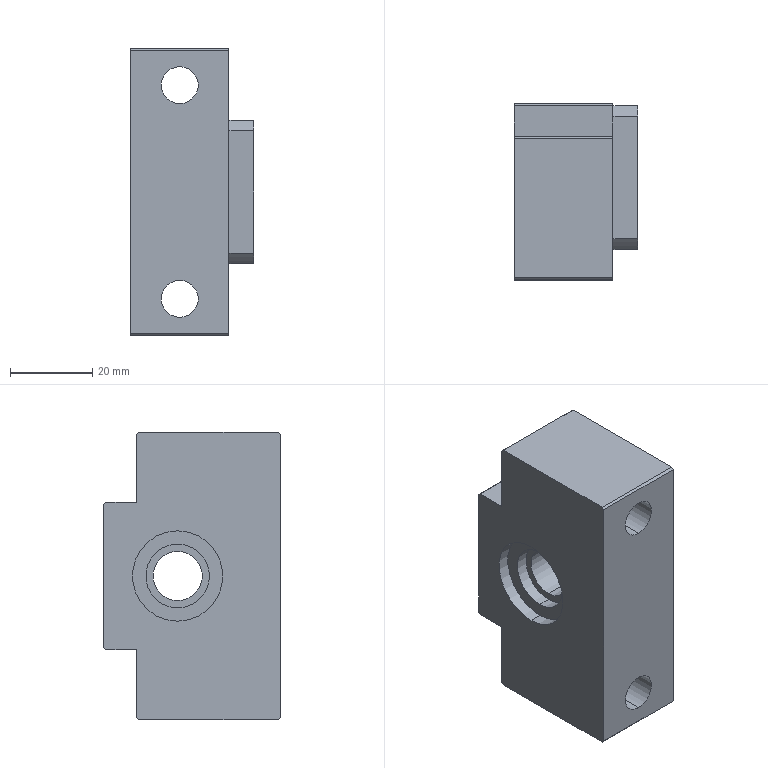Part | SolidWorks | features BaseBody 1 | 1 solid | 104 faces | box 30 x 43 x 70 mm | volume 59984 mm3 | plane 64 | cylinder 40 | commonest cylinder face diameters 7 x8 8 x8 9 x4 14 x4 15.5 x4 22 x4